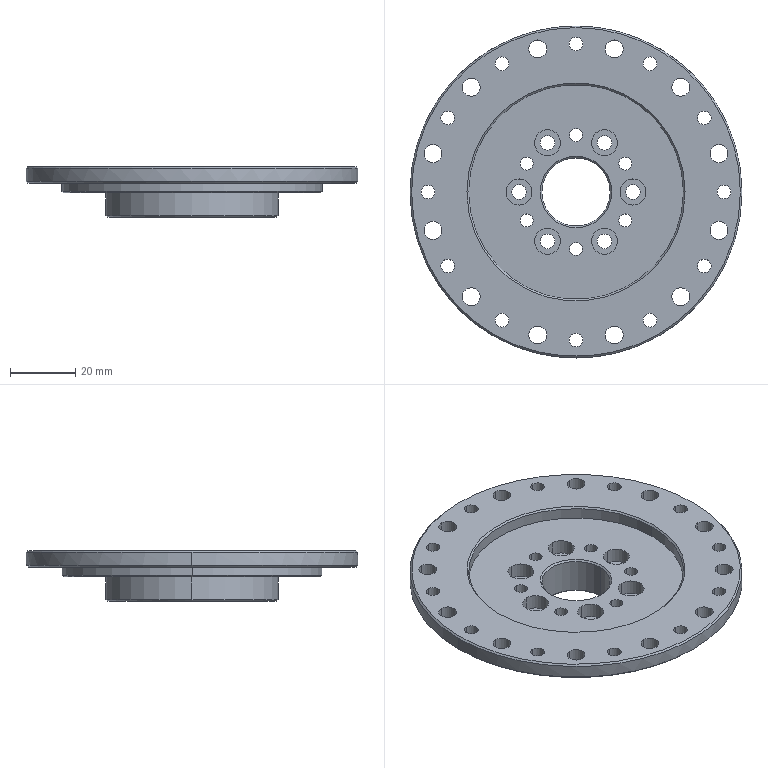Part | 1 solid | 122 faces | box 102 x 102 x 15.5 mm | volume 49476 mm3 | cylinder 94 | cone 17 | plane 11 | commonest cylinder face diameters 4.2 x24 5.5 x24 4 x12 4.5 x12 8 x12 21 x2